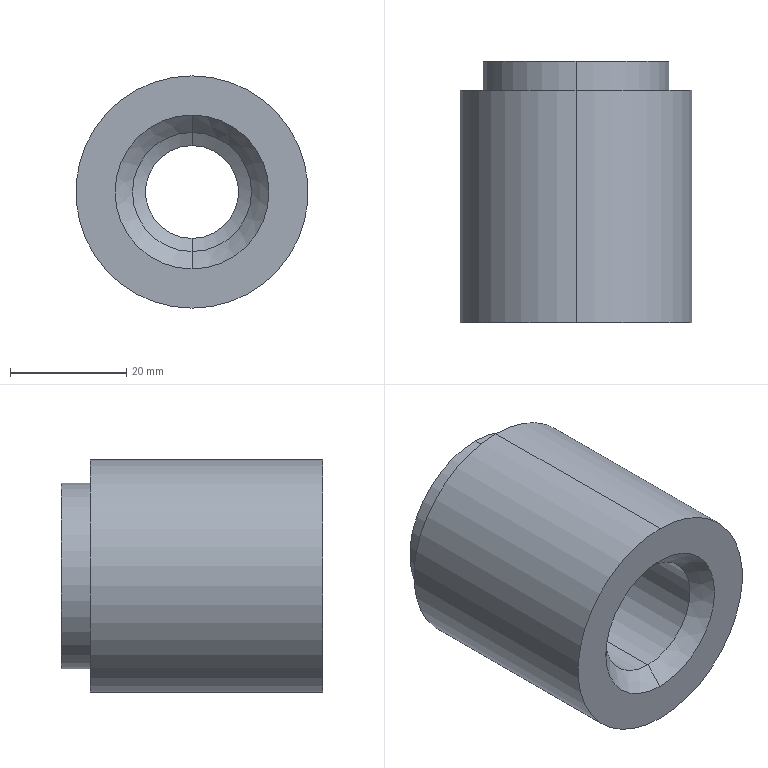Part | SolidWorks | features Chamfer 1, Revolution 1 | 1 solid | 15 faces | box 40 x 45 x 40 mm | volume 40970 mm3 | cylinder 8 | cone 4 | plane 3 | commonest cylinder face diameters 16 x2 20.5 x2 32 x2 40 x2
STEP:
#1=CARTESIAN_POINT('',(0.,3.,10.25));
#2=VERTEX_POINT('',#1);
#3=CARTESIAN_POINT('',(0.,3.,-10.25));
#4=VERTEX_POINT('',#3);
#5=CARTESIAN_POINT('',(0.,3.,0.));
#6=DIRECTION('',(0.,-1.,0.));
#7=DIRECTION('',(0.,0.,1.));
#8=AXIS2_PLACEMENT_3D('',#5,#6,#7);
#9=CIRCLE('',#8,10.25);
#10=EDGE_CURVE('',#2,#4,#9,.T.);
#11=ORIENTED_EDGE('',*,*,#10,.F.);
#12=CARTESIAN_POINT('',(0.,0.,13.25));
#13=VERTEX_POINT('',#12);
#14=CARTESIAN_POINT('',(0.,0.,13.25));
#15=DIRECTION('',(0.,-0.7071,0.7071));
#16=VECTOR('',#15,1000.);
#17=LINE('',#14,#16);
#18=EDGE_CURVE('',#2,#13,#17,.T.);
#19=ORIENTED_EDGE('',*,*,#18,.T.);
#20=CARTESIAN_POINT('',(0.,0.,-13.25));
#21=VERTEX_POINT('',#20);
#22=CARTESIAN_POINT('',(0.,0.,0.));
#23=DIRECTION('',(0.,1.,0.));
#24=DIRECTION('',(0.,0.,1.));
#25=AXIS2_PLACEMENT_3D('',#22,#23,#24);
#26=CIRCLE('',#25,13.25);
#27=EDGE_CURVE('',#21,#13,#26,.T.);
#28=ORIENTED_EDGE('',*,*,#27,.F.);
#29=CARTESIAN_POINT('',(0.,0.,-13.25));
#30=DIRECTION('',(0.,-0.7071,-0.7071));
#31=VECTOR('',#30,1000.);
#32=LINE('',#29,#31);
#33=EDGE_CURVE('',#4,#21,#32,.T.);
#34=ORIENTED_EDGE('',*,*,#33,.F.);
#35=EDGE_LOOP('',(#11,#19,#28,#34));
#36=FACE_OUTER_BOUND('',#35,.T.);
#37=CARTESIAN_POINT('',(0.,0.,0.));
#38=DIRECTION('',(0.,-1.,0.));
#39=DIRECTION('',(0.,0.,-1.));
#40=AXIS2_PLACEMENT_3D('',#37,#38,#39);
#41=CONICAL_SURFACE('',#40,13.25,0.7854);
#42=ADVANCED_FACE('',(#36),#41,.F.);
#43=ORIENTED_EDGE('',*,*,#10,.T.);
#44=CARTESIAN_POINT('',(0.,30.,-10.25));
#45=VERTEX_POINT('',#44);
#46=CARTESIAN_POINT('',(0.,45.,-10.25));
#47=DIRECTION('',(0.,1.,0.));
#48=VECTOR('',#47,1000.);
#49=LINE('',#46,#48);
#50=EDGE_CURVE('',#4,#45,#49,.T.);
#51=ORIENTED_EDGE('',*,*,#50,.T.);
#52=CARTESIAN_POINT('',(0.,30.,10.25));
#53=VERTEX_POINT('',#52);
#54=CARTESIAN_POINT('',(0.,30.,0.));
#55=DIRECTION('',(0.,1.,0.));
#56=DIRECTION('',(0.,0.,1.));
#57=AXIS2_PLACEMENT_3D('',#54,#55,#56);
#58=CIRCLE('',#57,10.25);
#59=EDGE_CURVE('',#45,#53,#58,.T.);
#60=ORIENTED_EDGE('',*,*,#59,.T.);
#61=CARTESIAN_POINT('',(0.,45.,10.25));
#62=DIRECTION('',(0.,1.,0.));
#63=VECTOR('',#62,1000.);
#64=LINE('',#61,#63);
#65=EDGE_CURVE('',#2,#53,#64,.T.);
#66=ORIENTED_EDGE('',*,*,#65,.F.);
#67=EDGE_LOOP('',(#43,#51,#60,#66));
#68=FACE_OUTER_BOUND('',#67,.T.);
#69=CARTESIAN_POINT('',(0.,45.,0.));
#70=DIRECTION('',(0.,1.,0.));
#71=DIRECTION('',(0.,0.,1.));
#72=AXIS2_PLACEMENT_3D('',#69,#70,#71);
#73=CYLINDRICAL_SURFACE('',#72,10.25);
#74=ADVANCED_FACE('',(#68),#73,.F.);
#75=CARTESIAN_POINT('',(0.,31.299,-8.));
#76=VERTEX_POINT('',#75);
#77=CARTESIAN_POINT('',(0.,31.299,8.));
#78=VERTEX_POINT('',#77);
#79=CARTESIAN_POINT('',(0.,31.299,0.));
#80=DIRECTION('',(0.,1.,0.));
#81=DIRECTION('',(0.,0.,1.));
#82=AXIS2_PLACEMENT_3D('',#79,#80,#81);
#83=CIRCLE('',#82,8.);
#84=EDGE_CURVE('',#76,#78,#83,.T.);
#85=ORIENTED_EDGE('',*,*,#84,.T.);
#86=CARTESIAN_POINT('',(0.,31.299,8.));
#87=DIRECTION('',(0.,-0.5,0.866));
#88=VECTOR('',#87,1000.);
#89=LINE('',#86,#88);
#90=EDGE_CURVE('',#78,#53,#89,.T.);
#91=ORIENTED_EDGE('',*,*,#90,.T.);
#92=ORIENTED_EDGE('',*,*,#59,.F.);
#93=CARTESIAN_POINT('',(0.,31.299,-8.));
#94=DIRECTION('',(0.,-0.5,-0.866));
#95=VECTOR('',#94,1000.);
#96=LINE('',#93,#95);
#97=EDGE_CURVE('',#76,#45,#96,.T.);
#98=ORIENTED_EDGE('',*,*,#97,.F.);
#99=EDGE_LOOP('',(#85,#91,#92,#98));
#100=FACE_OUTER_BOUND('',#99,.T.);
#101=CARTESIAN_POINT('',(0.,31.299,0.));
#102=DIRECTION('',(0.,-1.,0.));
#103=DIRECTION('',(0.,0.,-1.));
#104=AXIS2_PLACEMENT_3D('',#101,#102,#103);
#105=CONICAL_SURFACE('',#104,8.,1.047);
#106=ADVANCED_FACE('',(#100),#105,.F.);
#107=ORIENTED_EDGE('',*,*,#84,.F.);
#108=CARTESIAN_POINT('',(0.,45.,-8.));
#109=VERTEX_POINT('',#108);
#110=CARTESIAN_POINT('',(0.,45.,-8.));
#111=DIRECTION('',(0.,1.,0.));
#112=VECTOR('',#111,1000.);
#113=LINE('',#110,#112);
#114=EDGE_CURVE('',#76,#109,#113,.T.);
#115=ORIENTED_EDGE('',*,*,#114,.T.);
#116=CARTESIAN_POINT('',(0.,45.,8.));
#117=VERTEX_POINT('',#116);
#118=CARTESIAN_POINT('',(0.,45.,0.));
#119=DIRECTION('',(0.,1.,0.));
#120=DIRECTION('',(0.,0.,1.));
#121=AXIS2_PLACEMENT_3D('',#118,#119,#120);
#122=CIRCLE('',#121,8.);
#123=EDGE_CURVE('',#109,#117,#122,.T.);
#124=ORIENTED_EDGE('',*,*,#123,.T.);
#125=CARTESIAN_POINT('',(0.,45.,8.));
#126=DIRECTION('',(0.,1.,0.));
#127=VECTOR('',#126,1000.);
#128=LINE('',#125,#127);
#129=EDGE_CURVE('',#78,#117,#128,.T.);
#130=ORIENTED_EDGE('',*,*,#129,.F.);
#131=EDGE_LOOP('',(#107,#115,#124,#130));
#132=FACE_OUTER_BOUND('',#131,.T.);
#133=CARTESIAN_POINT('',(0.,45.,0.));
#134=DIRECTION('',(0.,1.,0.));
#135=DIRECTION('',(0.,0.,1.));
#136=AXIS2_PLACEMENT_3D('',#133,#134,#135);
#137=CYLINDRICAL_SURFACE('',#136,8.);
#138=ADVANCED_FACE('',(#132),#137,.F.);
#139=CARTESIAN_POINT('',(0.,40.,16.));
#140=VERTEX_POINT('',#139);
#141=CARTESIAN_POINT('',(0.,40.,-16.));
#142=VERTEX_POINT('',#141);
#143=CARTESIAN_POINT('',(0.,40.,0.));
#144=DIRECTION('',(0.,1.,0.));
#145=DIRECTION('',(0.,0.,1.));
#146=AXIS2_PLACEMENT_3D('',#143,#144,#145);
#147=CIRCLE('',#146,16.);
#148=EDGE_CURVE('',#140,#142,#147,.T.);
#149=ORIENTED_EDGE('',*,*,#148,.T.);
#150=CARTESIAN_POINT('',(0.,45.,-16.));
#151=VERTEX_POINT('',#150);
#152=CARTESIAN_POINT('',(0.,45.,-16.));
#153=DIRECTION('',(0.,1.,0.));
#154=VECTOR('',#153,1000.);
#155=LINE('',#152,#154);
#156=EDGE_CURVE('',#142,#151,#155,.T.);
#157=ORIENTED_EDGE('',*,*,#156,.T.);
#158=CARTESIAN_POINT('',(0.,45.,16.));
#159=VERTEX_POINT('',#158);
#160=CARTESIAN_POINT('',(0.,45.,0.));
#161=DIRECTION('',(0.,1.,0.));
#162=DIRECTION('',(0.,0.,1.));
#163=AXIS2_PLACEMENT_3D('',#160,#161,#162);
#164=CIRCLE('',#163,16.);
#165=EDGE_CURVE('',#159,#151,#164,.T.);
#166=ORIENTED_EDGE('',*,*,#165,.F.);
#167=CARTESIAN_POINT('',(0.,45.,16.));
#168=DIRECTION('',(0.,1.,0.));
#169=VECTOR('',#168,1000.);
#170=LINE('',#167,#169);
#171=EDGE_CURVE('',#140,#159,#170,.T.);
#172=ORIENTED_EDGE('',*,*,#171,.F.);
#173=EDGE_LOOP('',(#149,#157,#166,#172));
#174=FACE_OUTER_BOUND('',#173,.T.);
#175=CARTESIAN_POINT('',(0.,45.,0.));
#176=DIRECTION('',(0.,1.,0.));
#177=DIRECTION('',(0.,0.,1.));
#178=AXIS2_PLACEMENT_3D('',#175,#176,#177);
#179=CYLINDRICAL_SURFACE('',#178,16.);
#180=ADVANCED_FACE('',(#174),#179,.T.);
#181=CARTESIAN_POINT('',(0.,0.,20.));
#182=VERTEX_POINT('',#181);
#183=CARTESIAN_POINT('',(0.,0.,-20.));
#184=VERTEX_POINT('',#183);
#185=CARTESIAN_POINT('',(0.,0.,0.));
#186=DIRECTION('',(0.,1.,0.));
#187=DIRECTION('',(0.,0.,1.));
#188=AXIS2_PLACEMENT_3D('',#185,#186,#187);
#189=CIRCLE('',#188,20.);
#190=EDGE_CURVE('',#182,#184,#189,.T.);
#191=ORIENTED_EDGE('',*,*,#190,.T.);
#192=CARTESIAN_POINT('',(0.,40.,-20.));
#193=VERTEX_POINT('',#192);
#194=CARTESIAN_POINT('',(0.,45.,-20.));
#195=DIRECTION('',(0.,1.,0.));
#196=VECTOR('',#195,1000.);
#197=LINE('',#194,#196);
#198=EDGE_CURVE('',#184,#193,#197,.T.);
#199=ORIENTED_EDGE('',*,*,#198,.T.);
#200=CARTESIAN_POINT('',(0.,40.,20.));
#201=VERTEX_POINT('',#200);
#202=CARTESIAN_POINT('',(0.,40.,0.));
#203=DIRECTION('',(0.,1.,0.));
#204=DIRECTION('',(0.,0.,1.));
#205=AXIS2_PLACEMENT_3D('',#202,#203,#204);
#206=CIRCLE('',#205,20.);
#207=EDGE_CURVE('',#201,#193,#206,.T.);
#208=ORIENTED_EDGE('',*,*,#207,.F.);
#209=CARTESIAN_POINT('',(0.,45.,20.));
#210=DIRECTION('',(0.,1.,0.));
#211=VECTOR('',#210,1000.);
#212=LINE('',#209,#211);
#213=EDGE_CURVE('',#182,#201,#212,.T.);
#214=ORIENTED_EDGE('',*,*,#213,.F.);
#215=EDGE_LOOP('',(#191,#199,#208,#214));
#216=FACE_OUTER_BOUND('',#215,.T.);
#217=CARTESIAN_POINT('',(0.,45.,0.));
#218=DIRECTION('',(0.,1.,0.));
#219=DIRECTION('',(0.,0.,1.));
#220=AXIS2_PLACEMENT_3D('',#217,#218,#219);
#221=CYLINDRICAL_SURFACE('',#220,20.);
#222=ADVANCED_FACE('',(#216),#221,.T.);
#223=ORIENTED_EDGE('',*,*,#198,.F.);
#224=CARTESIAN_POINT('',(0.,0.,0.));
#225=DIRECTION('',(0.,1.,0.));
#226=DIRECTION('',(0.,0.,1.));
#227=AXIS2_PLACEMENT_3D('',#224,#225,#226);
#228=CIRCLE('',#227,20.);
#229=EDGE_CURVE('',#184,#182,#228,.T.);
#230=ORIENTED_EDGE('',*,*,#229,.T.);
#231=ORIENTED_EDGE('',*,*,#213,.T.);
#232=CARTESIAN_POINT('',(0.,40.,0.));
#233=DIRECTION('',(0.,1.,0.));
#234=DIRECTION('',(0.,0.,1.));
#235=AXIS2_PLACEMENT_3D('',#232,#233,#234);
#236=CIRCLE('',#235,20.);
#237=EDGE_CURVE('',#193,#201,#236,.T.);
#238=ORIENTED_EDGE('',*,*,#237,.F.);
#239=EDGE_LOOP('',(#223,#230,#231,#238));
#240=FACE_OUTER_BOUND('',#239,.T.);
#241=CARTESIAN_POINT('',(0.,45.,0.));
#242=DIRECTION('',(0.,1.,0.));
#243=DIRECTION('',(0.,0.,1.));
#244=AXIS2_PLACEMENT_3D('',#241,#242,#243);
#245=CYLINDRICAL_SURFACE('',#244,20.);
#246=ADVANCED_FACE('',(#240),#245,.T.);
#247=ORIENTED_EDGE('',*,*,#148,.F.);
#248=CARTESIAN_POINT('',(0.,40.,0.));
#249=DIRECTION('',(0.,1.,0.));
#250=DIRECTION('',(0.,0.,1.));
#251=AXIS2_PLACEMENT_3D('',#248,#249,#250);
#252=CIRCLE('',#251,16.);
#253=EDGE_CURVE('',#142,#140,#252,.T.);
#254=ORIENTED_EDGE('',*,*,#253,.F.);
#255=EDGE_LOOP('',(#247,#254));
#256=FACE_BOUND('',#255,.T.);
#257=ORIENTED_EDGE('',*,*,#207,.T.);
#258=ORIENTED_EDGE('',*,*,#237,.T.);
#259=EDGE_LOOP('',(#257,#258));
#260=FACE_OUTER_BOUND('',#259,.T.);
#261=CARTESIAN_POINT('',(20.,40.,0.));
#262=DIRECTION('',(0.,-1.,0.));
#263=DIRECTION('',(0.,0.,-1.));
#264=AXIS2_PLACEMENT_3D('',#261,#262,#263);
#265=PLANE('',#264);
#266=ADVANCED_FACE('',(#256,#260),#265,.F.);
#267=ORIENTED_EDGE('',*,*,#156,.F.);
#268=ORIENTED_EDGE('',*,*,#253,.T.);
#269=ORIENTED_EDGE('',*,*,#171,.T.);
#270=CARTESIAN_POINT('',(0.,45.,0.));
#271=DIRECTION('',(0.,1.,0.));
#272=DIRECTION('',(0.,0.,1.));
#273=AXIS2_PLACEMENT_3D('',#270,#271,#272);
#274=CIRCLE('',#273,16.);
#275=EDGE_CURVE('',#151,#159,#274,.T.);
#276=ORIENTED_EDGE('',*,*,#275,.F.);
#277=EDGE_LOOP('',(#267,#268,#269,#276));
#278=FACE_OUTER_BOUND('',#277,.T.);
#279=CARTESIAN_POINT('',(0.,45.,0.));
#280=DIRECTION('',(0.,1.,0.));
#281=DIRECTION('',(0.,0.,1.));
#282=AXIS2_PLACEMENT_3D('',#279,#280,#281);
#283=CYLINDRICAL_SURFACE('',#282,16.);
#284=ADVANCED_FACE('',(#278),#283,.T.);
#285=CARTESIAN_POINT('',(0.,45.,0.));
#286=DIRECTION('',(0.,1.,0.));
#287=DIRECTION('',(0.,0.,1.));
#288=AXIS2_PLACEMENT_3D('',#285,#286,#287);
#289=CIRCLE('',#288,8.);
#290=EDGE_CURVE('',#117,#109,#289,.T.);
#291=ORIENTED_EDGE('',*,*,#290,.F.);
#292=ORIENTED_EDGE('',*,*,#123,.F.);
#293=EDGE_LOOP('',(#291,#292));
#294=FACE_BOUND('',#293,.T.);
#295=ORIENTED_EDGE('',*,*,#165,.T.);
#296=ORIENTED_EDGE('',*,*,#275,.T.);
#297=EDGE_LOOP('',(#295,#296));
#298=FACE_OUTER_BOUND('',#297,.T.);
#299=CARTESIAN_POINT('',(16.,45.,0.));
#300=DIRECTION('',(0.,-1.,0.));
#301=DIRECTION('',(0.,0.,-1.));
#302=AXIS2_PLACEMENT_3D('',#299,#300,#301);
#303=PLANE('',#302);
#304=ADVANCED_FACE('',(#294,#298),#303,.F.);
#305=ORIENTED_EDGE('',*,*,#114,.F.);
#306=CARTESIAN_POINT('',(0.,31.299,0.));
#307=DIRECTION('',(0.,1.,0.));
#308=DIRECTION('',(0.,0.,1.));
#309=AXIS2_PLACEMENT_3D('',#306,#307,#308);
#310=CIRCLE('',#309,8.);
#311=EDGE_CURVE('',#78,#76,#310,.T.);
#312=ORIENTED_EDGE('',*,*,#311,.F.);
#313=ORIENTED_EDGE('',*,*,#129,.T.);
#314=ORIENTED_EDGE('',*,*,#290,.T.);
#315=EDGE_LOOP('',(#305,#312,#313,#314));
#316=FACE_OUTER_BOUND('',#315,.T.);
#317=CARTESIAN_POINT('',(0.,45.,0.));
#318=DIRECTION('',(0.,1.,0.));
#319=DIRECTION('',(0.,0.,1.));
#320=AXIS2_PLACEMENT_3D('',#317,#318,#319);
#321=CYLINDRICAL_SURFACE('',#320,8.);
#322=ADVANCED_FACE('',(#316),#321,.F.);
#323=ORIENTED_EDGE('',*,*,#90,.F.);
#324=ORIENTED_EDGE('',*,*,#311,.T.);
#325=ORIENTED_EDGE('',*,*,#97,.T.);
#326=CARTESIAN_POINT('',(0.,30.,0.));
#327=DIRECTION('',(0.,1.,0.));
#328=DIRECTION('',(0.,0.,1.));
#329=AXIS2_PLACEMENT_3D('',#326,#327,#328);
#330=CIRCLE('',#329,10.25);
#331=EDGE_CURVE('',#53,#45,#330,.T.);
#332=ORIENTED_EDGE('',*,*,#331,.F.);
#333=EDGE_LOOP('',(#323,#324,#325,#332));
#334=FACE_OUTER_BOUND('',#333,.T.);
#335=CARTESIAN_POINT('',(0.,31.299,0.));
#336=DIRECTION('',(0.,-1.,0.));
#337=DIRECTION('',(0.,0.,-1.));
#338=AXIS2_PLACEMENT_3D('',#335,#336,#337);
#339=CONICAL_SURFACE('',#338,8.,1.047);
#340=ADVANCED_FACE('',(#334),#339,.F.);
#341=ORIENTED_EDGE('',*,*,#50,.F.);
#342=CARTESIAN_POINT('',(0.,3.,0.));
#343=DIRECTION('',(0.,-1.,0.));
#344=DIRECTION('',(0.,0.,1.));
#345=AXIS2_PLACEMENT_3D('',#342,#343,#344);
#346=CIRCLE('',#345,10.25);
#347=EDGE_CURVE('',#4,#2,#346,.T.);
#348=ORIENTED_EDGE('',*,*,#347,.T.);
#349=ORIENTED_EDGE('',*,*,#65,.T.);
#350=ORIENTED_EDGE('',*,*,#331,.T.);
#351=EDGE_LOOP('',(#341,#348,#349,#350));
#352=FACE_OUTER_BOUND('',#351,.T.);
#353=CARTESIAN_POINT('',(0.,45.,0.));
#354=DIRECTION('',(0.,1.,0.));
#355=DIRECTION('',(0.,0.,1.));
#356=AXIS2_PLACEMENT_3D('',#353,#354,#355);
#357=CYLINDRICAL_SURFACE('',#356,10.25);
#358=ADVANCED_FACE('',(#352),#357,.F.);
#359=ORIENTED_EDGE('',*,*,#27,.T.);
#360=CARTESIAN_POINT('',(0.,0.,0.));
#361=DIRECTION('',(0.,1.,0.));
#362=DIRECTION('',(0.,0.,1.));
#363=AXIS2_PLACEMENT_3D('',#360,#361,#362);
#364=CIRCLE('',#363,13.25);
#365=EDGE_CURVE('',#13,#21,#364,.T.);
#366=ORIENTED_EDGE('',*,*,#365,.T.);
#367=EDGE_LOOP('',(#359,#366));
#368=FACE_BOUND('',#367,.T.);
#369=ORIENTED_EDGE('',*,*,#190,.F.);
#370=ORIENTED_EDGE('',*,*,#229,.F.);
#371=EDGE_LOOP('',(#369,#370));
#372=FACE_OUTER_BOUND('',#371,.T.);
#373=CARTESIAN_POINT('',(10.25,0.,0.));
#374=DIRECTION('',(0.,1.,0.));
#375=DIRECTION('',(0.,0.,1.));
#376=AXIS2_PLACEMENT_3D('',#373,#374,#375);
#377=PLANE('',#376);
#378=ADVANCED_FACE('',(#368,#372),#377,.F.);
#379=ORIENTED_EDGE('',*,*,#18,.F.);
#380=ORIENTED_EDGE('',*,*,#347,.F.);
#381=ORIENTED_EDGE('',*,*,#33,.T.);
#382=ORIENTED_EDGE('',*,*,#365,.F.);
#383=EDGE_LOOP('',(#379,#380,#381,#382));
#384=FACE_OUTER_BOUND('',#383,.T.);
#385=CARTESIAN_POINT('',(0.,0.,0.));
#386=DIRECTION('',(0.,-1.,0.));
#387=DIRECTION('',(0.,0.,-1.));
#388=AXIS2_PLACEMENT_3D('',#385,#386,#387);
#389=CONICAL_SURFACE('',#388,13.25,0.7854);
#390=ADVANCED_FACE('',(#384),#389,.F.);
#391=CLOSED_SHELL('',(#42,#74,#106,#138,#180,#222,#246,#266,#284,#304,#322,#340,#358,#378,#390));
#392=MANIFOLD_SOLID_BREP('',#391);
#393=CARTESIAN_POINT('',(0.,0.,0.));
#394=DIRECTION('',(0.,0.,1.));
#395=DIRECTION('',(1.,0.,0.));
#396=AXIS2_PLACEMENT_3D('',#393,#394,#395);
#397=(LENGTH_UNIT()NAMED_UNIT(*)SI_UNIT(.MILLI.,.METRE.));
#398=UNCERTAINTY_MEASURE_WITH_UNIT(LENGTH_MEASURE(0.00001),#397,'','');
#399=(NAMED_UNIT(*)PLANE_ANGLE_UNIT()SI_UNIT($,.RADIAN.));
#400=(NAMED_UNIT(*)SI_UNIT($,.STERADIAN.)SOLID_ANGLE_UNIT());
#401=(GEOMETRIC_REPRESENTATION_CONTEXT(3)GLOBAL_UNCERTAINTY_ASSIGNED_CONTEXT((#398))GLOBAL_UNIT_ASSIGNED_CONTEXT((#397,#399,#400))REPRESENTATION_CONTEXT('',''));
#402=ADVANCED_BREP_SHAPE_REPRESENTATION('',(#392,#396),#401);